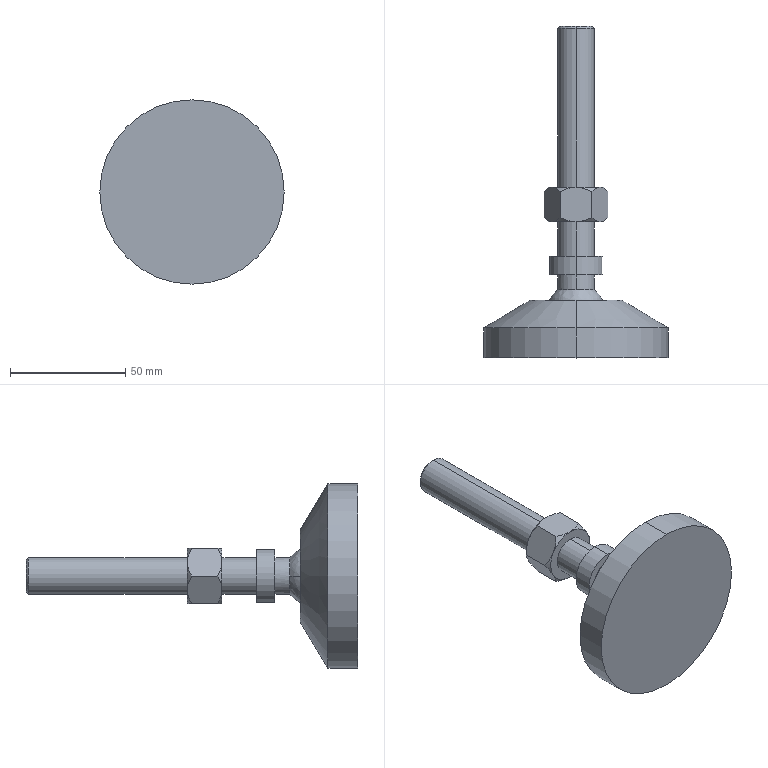Part | STEP file | 2 solids | 43 faces | box 80 x 144 x 80 mm | volume 131101 mm3 | cone 16 | plane 13 | cylinder 10 | spline 4 | commonest cylinder face diameters 16 x6 23 x2 80 x2